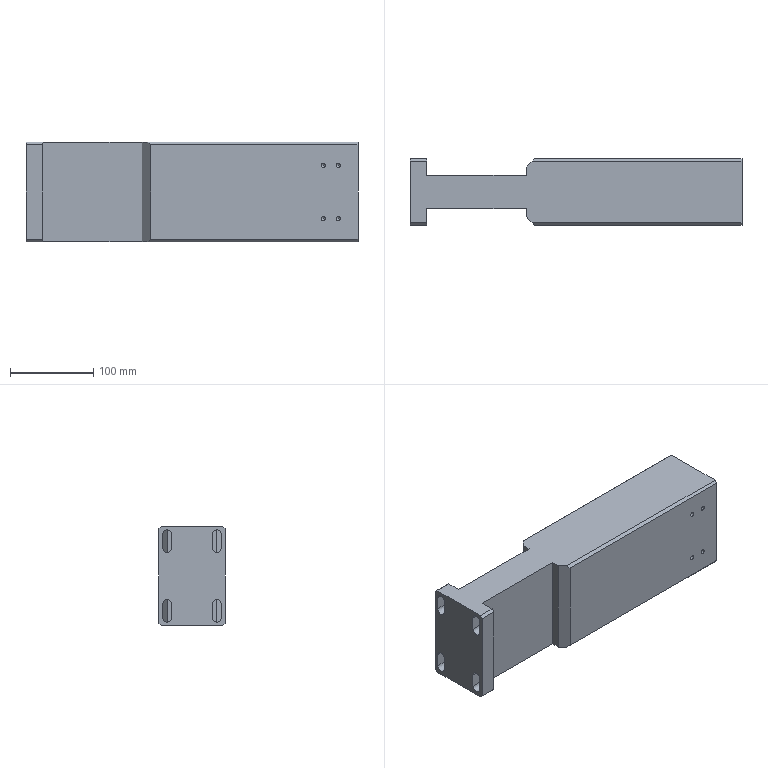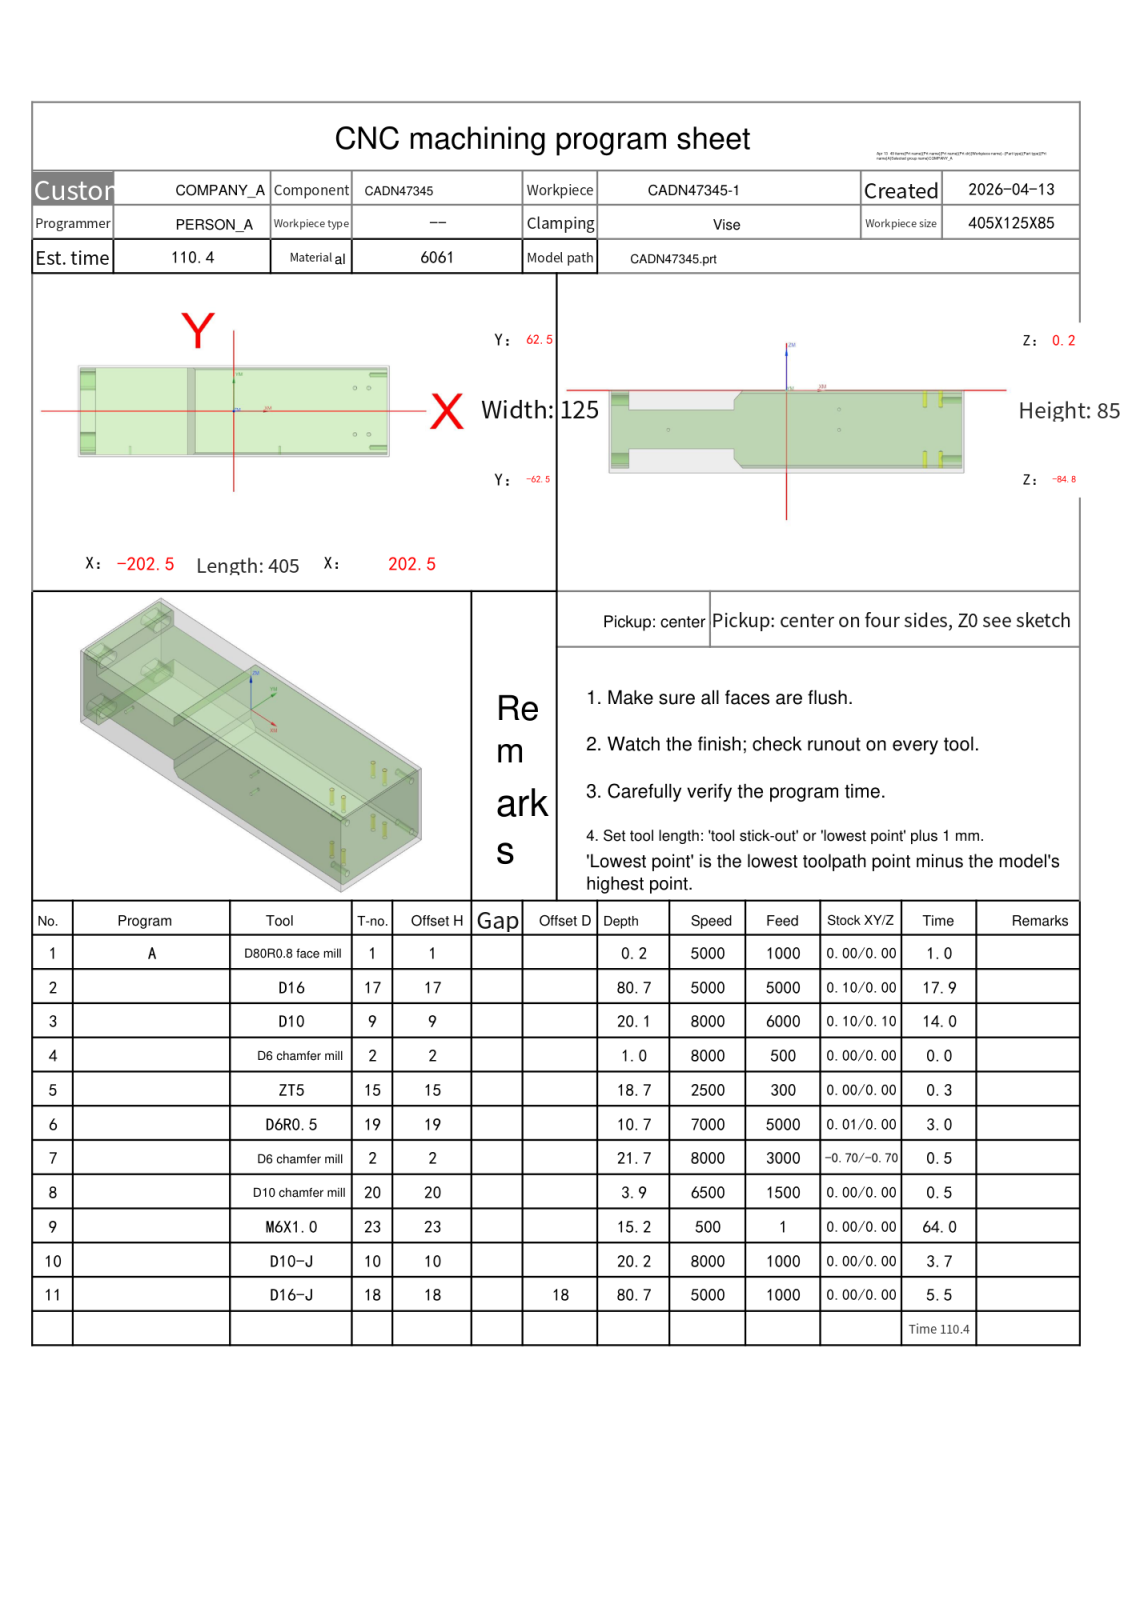NC program | NX | posted by the shop | part box 400 x 80 x 120 mm
Lines 1 to 710 of 5986:
%
O0001
(Machine time: 172.73 MIN)
(===Total Tool:10===)
(T1=D80R0.8 face mill D=80.  R=0.8  D-  H01 Z=0.    )
(T17=D16    D=16.  R=0.   D-  H17 Z=-80.5 )
(T9=D10     D=10.  R=0.   D-  H09 Z=-19.9 )
(T2=D6 chamfer mill   D=6.   R=0.   D-  H02 Z=-21.5 )
(T15=ZT5    D=5.   DR_a=118 D-  H15 Z=-18.5 )
(T19=D6R0.5 D=6.   R=0.5  D-  H19 Z=-10.5 )
(T20=D10 chamfer mill D=10.  R=0.  D-  H20 Z=-3.7  )
(T23=M6X1.0 D=5.   DR_a=180 D-  H23 Z=-15.  )
(T10=D10-J  D=10.  R=0.   D10 H10 Z=-20.  )
(T18=D16-J  D=16.  R=0.   D18 H18 Z=-80.5 )
G80 G90 G17 G49 G40
G91 G28 Z0
M01
N1 T01 M06
(D80R0.8 face mill  D=80. R=0.8 H=01 ce=0.00 di=0.00)
G00 G90 G54 X245. Y-33.333 M03 S5000
G43 H01 Z20.
M08
Z2.
G01 Z0.0 F1000.
X240.
X-240.
Y33.333
X240.
X245.
Z2.
G00 Z20.
G91 G28 Z0.0
M05
M09
G91 G28 Z0.0
M01
N2 T17 M06
(D16  D=16. R=0. H=17 ce=0.10 di=0.00)
G00 G90 G54 X0.0 Y68.1 M03 S5000
G43 H17 Z20.
M08
Z.5
G01 X200. Z.317 F5000.
G02 X208.1 Y60. Z.305 I0.0 J-8.1
G01 Y-60. Z.195
G02 X200. Y-68.1 Z.183 I-8.1 J0.0
G01 X-200. Z-.183
G02 X-208.1 Y-60. Z-.195 I0.0 J8.1
G01 Y60. Z-.305
G02 X-200. Y68.1 Z-.317 I8.1 J0.0
G01 X200. Z-.683
G02 X208.1 Y60. Z-.695 I0.0 J-8.1
G01 Y-60. Z-.805
G02 X200. Y-68.1 Z-.817 I-8.1 J0.0
G01 X-200. Z-1.183
G02 X-208.1 Y-60. Z-1.195 I0.0 J8.1
G01 Y60. Z-1.305
G02 X-200. Y68.1 Z-1.317 I8.1 J0.0
G01 X200. Z-1.683
G02 X208.1 Y60. Z-1.695 I0.0 J-8.1
G01 Y-60. Z-1.805
G02 X200. Y-68.1 Z-1.817 I-8.1 J0.0
G01 X-200. Z-2.183
G02 X-208.1 Y-60. Z-2.195 I0.0 J8.1
G01 Y60. Z-2.305
G02 X-200. Y68.1 Z-2.317 I8.1 J0.0
G01 X200. Z-2.683
G02 X208.1 Y60. Z-2.695 I0.0 J-8.1
G01 Y-60. Z-2.805
G02 X200. Y-68.1 Z-2.817 I-8.1 J0.0
G01 X-200. Z-3.183
G02 X-208.1 Y-60. Z-3.195 I0.0 J8.1
G01 Y60. Z-3.305
G02 X-200. Y68.1 Z-3.317 I8.1 J0.0
G01 X200. Z-3.683
G02 X208.1 Y60. Z-3.695 I0.0 J-8.1
G01 Y-60. Z-3.805
G02 X200. Y-68.1 Z-3.817 I-8.1 J0.0
G01 X-200. Z-4.183
G02 X-208.1 Y-60. Z-4.195 I0.0 J8.1
G01 Y60. Z-4.305
G02 X-200. Y68.1 Z-4.317 I8.1 J0.0
G01 X200. Z-4.683
G02 X208.1 Y60. Z-4.695 I0.0 J-8.1
G01 Y-60. Z-4.805
G02 X200. Y-68.1 Z-4.817 I-8.1 J0.0
G01 X-200. Z-5.183
G02 X-208.1 Y-60. Z-5.195 I0.0 J8.1
G01 Y60. Z-5.305
G02 X-200. Y68.1 Z-5.317 I8.1 J0.0
G01 X200. Z-5.683
G02 X208.1 Y60. Z-5.695 I0.0 J-8.1
G01 Y-60. Z-5.805
G02 X200. Y-68.1 Z-5.817 I-8.1 J0.0
G01 X-200. Z-6.183
G02 X-208.1 Y-60. Z-6.195 I0.0 J8.1
G01 Y60. Z-6.305
G02 X-200. Y68.1 Z-6.317 I8.1 J0.0
G01 X200. Z-6.683
G02 X208.1 Y60. Z-6.695 I0.0 J-8.1
G01 Y-60. Z-6.805
G02 X200. Y-68.1 Z-6.817 I-8.1 J0.0
G01 X-200. Z-7.183
G02 X-208.1 Y-60. Z-7.195 I0.0 J8.1
G01 Y60. Z-7.305
G02 X-200. Y68.1 Z-7.317 I8.1 J0.0
G01 X200. Z-7.683
G02 X208.1 Y60. Z-7.695 I0.0 J-8.1
G01 Y-60. Z-7.805
G02 X200. Y-68.1 Z-7.817 I-8.1 J0.0
G01 X-200. Z-8.183
G02 X-208.1 Y-60. Z-8.195 I0.0 J8.1
G01 Y60. Z-8.305
G02 X-200. Y68.1 Z-8.317 I8.1 J0.0
G01 X200. Z-8.683
G02 X208.1 Y60. Z-8.695 I0.0 J-8.1
G01 Y-60. Z-8.805
G02 X200. Y-68.1 Z-8.817 I-8.1 J0.0
G01 X-200. Z-9.183
G02 X-208.1 Y-60. Z-9.195 I0.0 J8.1
G01 Y60. Z-9.305
G02 X-200. Y68.1 Z-9.317 I8.1 J0.0
G01 X200. Z-9.683
G02 X208.1 Y60. Z-9.695 I0.0 J-8.1
G01 Y-60. Z-9.805
G02 X200. Y-68.1 Z-9.817 I-8.1 J0.0
G01 X-200. Z-10.183
G02 X-208.1 Y-60. Z-10.195 I0.0 J8.1
G01 Y60. Z-10.305
G02 X-200. Y68.1 Z-10.317 I8.1 J0.0
G01 X200. Z-10.683
G02 X208.1 Y60. Z-10.695 I0.0 J-8.1
G01 Y-60. Z-10.805
G02 X200. Y-68.1 Z-10.817 I-8.1 J0.0
G01 X-200. Z-11.183
G02 X-208.1 Y-60. Z-11.195 I0.0 J8.1
G01 Y60. Z-11.305
G02 X-200. Y68.1 Z-11.317 I8.1 J0.0
G01 X200. Z-11.683
G02 X208.1 Y60. Z-11.695 I0.0 J-8.1
G01 Y-60. Z-11.805
G02 X200. Y-68.1 Z-11.817 I-8.1 J0.0
G01 X-200. Z-12.183
G02 X-208.1 Y-60. Z-12.195 I0.0 J8.1
G01 Y60. Z-12.305
G02 X-200. Y68.1 Z-12.317 I8.1 J0.0
G01 X200. Z-12.683
G02 X208.1 Y60. Z-12.695 I0.0 J-8.1
G01 Y-60. Z-12.805
G02 X200. Y-68.1 Z-12.817 I-8.1 J0.0
G01 X-200. Z-13.183
G02 X-208.1 Y-60. Z-13.195 I0.0 J8.1
G01 Y60. Z-13.305
G02 X-200. Y68.1 Z-13.317 I8.1 J0.0
G01 X200. Z-13.683
G02 X208.1 Y60. Z-13.695 I0.0 J-8.1
G01 Y-60. Z-13.805
G02 X200. Y-68.1 Z-13.817 I-8.1 J0.0
G01 X-200. Z-14.183
G02 X-208.1 Y-60. Z-14.195 I0.0 J8.1
G01 Y60. Z-14.305
G02 X-200. Y68.1 Z-14.317 I8.1 J0.0
G01 X200. Z-14.683
G02 X208.1 Y60. Z-14.695 I0.0 J-8.1
G01 Y-60. Z-14.805
G02 X200. Y-68.1 Z-14.817 I-8.1 J0.0
G01 X-200. Z-15.183
G02 X-208.1 Y-60. Z-15.195 I0.0 J8.1
G01 Y60. Z-15.305
G02 X-200. Y68.1 Z-15.317 I8.1 J0.0
G01 X200. Z-15.683
G02 X208.1 Y60. Z-15.695 I0.0 J-8.1
G01 Y-60. Z-15.805
G02 X200. Y-68.1 Z-15.817 I-8.1 J0.0
G01 X-200. Z-16.183
G02 X-208.1 Y-60. Z-16.195 I0.0 J8.1
G01 Y60. Z-16.305
G02 X-200. Y68.1 Z-16.317 I8.1 J0.0
G01 X200. Z-16.683
G02 X208.1 Y60. Z-16.695 I0.0 J-8.1
G01 Y-60. Z-16.805
G02 X200. Y-68.1 Z-16.817 I-8.1 J0.0
G01 X-200. Z-17.183
G02 X-208.1 Y-60. Z-17.195 I0.0 J8.1
G01 Y60. Z-17.305
G02 X-200. Y68.1 Z-17.317 I8.1 J0.0
G01 X200. Z-17.683
G02 X208.1 Y60. Z-17.695 I0.0 J-8.1
G01 Y-60. Z-17.805
G02 X200. Y-68.1 Z-17.817 I-8.1 J0.0
G01 X-200. Z-18.183
G02 X-208.1 Y-60. Z-18.195 I0.0 J8.1
G01 Y60. Z-18.305
G02 X-200. Y68.1 Z-18.317 I8.1 J0.0
G01 X200. Z-18.683
G02 X208.1 Y60. Z-18.695 I0.0 J-8.1
G01 Y-60. Z-18.805
G02 X200. Y-68.1 Z-18.817 I-8.1 J0.0
G01 X-200. Z-19.183
G02 X-208.1 Y-60. Z-19.195 I0.0 J8.1
G01 Y60. Z-19.305
G02 X-200. Y68.1 Z-19.317 I8.1 J0.0
G01 X200. Z-19.683
G02 X208.1 Y60. Z-19.695 I0.0 J-8.1
G01 Y-60. Z-19.805
G02 X200. Y-68.1 Z-19.817 I-8.1 J0.0
G01 X-200. Z-20.183
G02 X-208.1 Y-60. Z-20.195 I0.0 J8.1
G01 Y60. Z-20.305
G02 X-200. Y68.1 Z-20.317 I8.1 J0.0
G01 X200. Z-20.683
G02 X208.1 Y60. Z-20.695 I0.0 J-8.1
G01 Y-60. Z-20.805
G02 X200. Y-68.1 Z-20.817 I-8.1 J0.0
G01 X-200. Z-21.183
G02 X-208.1 Y-60. Z-21.195 I0.0 J8.1
G01 Y60. Z-21.305
G02 X-200. Y68.1 Z-21.317 I8.1 J0.0
G01 X200. Z-21.683
G02 X208.1 Y60. Z-21.695 I0.0 J-8.1
G01 Y-60. Z-21.805
G02 X200. Y-68.1 Z-21.817 I-8.1 J0.0
G01 X-200. Z-22.183
G02 X-208.1 Y-60. Z-22.195 I0.0 J8.1
G01 Y60. Z-22.305
G02 X-200. Y68.1 Z-22.317 I8.1 J0.0
G01 X200. Z-22.683
G02 X208.1 Y60. Z-22.695 I0.0 J-8.1
G01 Y-60. Z-22.805
G02 X200. Y-68.1 Z-22.817 I-8.1 J0.0
G01 X-200. Z-23.183
G02 X-208.1 Y-60. Z-23.195 I0.0 J8.1
G01 Y60. Z-23.305
G02 X-200. Y68.1 Z-23.317 I8.1 J0.0
G01 X200. Z-23.683
G02 X208.1 Y60. Z-23.695 I0.0 J-8.1
G01 Y-60. Z-23.805
G02 X200. Y-68.1 Z-23.817 I-8.1 J0.0
G01 X-200. Z-24.183
G02 X-208.1 Y-60. Z-24.195 I0.0 J8.1
G01 Y60. Z-24.305
G02 X-200. Y68.1 Z-24.317 I8.1 J0.0
G01 X200. Z-24.683
G02 X208.1 Y60. Z-24.695 I0.0 J-8.1
G01 Y-60. Z-24.805
G02 X200. Y-68.1 Z-24.817 I-8.1 J0.0
G01 X-200. Z-25.183
G02 X-208.1 Y-60. Z-25.195 I0.0 J8.1
G01 Y60. Z-25.305
G02 X-200. Y68.1 Z-25.317 I8.1 J0.0
G01 X200. Z-25.683
G02 X208.1 Y60. Z-25.695 I0.0 J-8.1
G01 Y-60. Z-25.805
G02 X200. Y-68.1 Z-25.817 I-8.1 J0.0
G01 X-200. Z-26.183
G02 X-208.1 Y-60. Z-26.195 I0.0 J8.1
G01 Y60. Z-26.305
G02 X-200. Y68.1 Z-26.317 I8.1 J0.0
G01 X200. Z-26.683
G02 X208.1 Y60. Z-26.695 I0.0 J-8.1
G01 Y-60. Z-26.805
G02 X200. Y-68.1 Z-26.817 I-8.1 J0.0
G01 X-200. Z-27.183
G02 X-208.1 Y-60. Z-27.195 I0.0 J8.1
G01 Y60. Z-27.305
G02 X-200. Y68.1 Z-27.317 I8.1 J0.0
G01 X200. Z-27.683
G02 X208.1 Y60. Z-27.695 I0.0 J-8.1
G01 Y-60. Z-27.805
G02 X200. Y-68.1 Z-27.817 I-8.1 J0.0
G01 X-200. Z-28.183
G02 X-208.1 Y-60. Z-28.195 I0.0 J8.1
G01 Y60. Z-28.305
G02 X-200. Y68.1 Z-28.317 I8.1 J0.0
G01 X200. Z-28.683
G02 X208.1 Y60. Z-28.695 I0.0 J-8.1
G01 Y-60. Z-28.805
G02 X200. Y-68.1 Z-28.817 I-8.1 J0.0
G01 X-200. Z-29.183
G02 X-208.1 Y-60. Z-29.195 I0.0 J8.1
G01 Y60. Z-29.305
G02 X-200. Y68.1 Z-29.317 I8.1 J0.0
G01 X200. Z-29.683
G02 X208.1 Y60. Z-29.695 I0.0 J-8.1
G01 Y-60. Z-29.805
G02 X200. Y-68.1 Z-29.817 I-8.1 J0.0
G01 X-200. Z-30.183
G02 X-208.1 Y-60. Z-30.195 I0.0 J8.1
G01 Y60. Z-30.305
G02 X-200. Y68.1 Z-30.317 I8.1 J0.0
G01 X200. Z-30.683
G02 X208.1 Y60. Z-30.695 I0.0 J-8.1
G01 Y-60. Z-30.805
G02 X200. Y-68.1 Z-30.817 I-8.1 J0.0
G01 X-200. Z-31.183
G02 X-208.1 Y-60. Z-31.195 I0.0 J8.1
G01 Y60. Z-31.305
G02 X-200. Y68.1 Z-31.317 I8.1 J0.0
G01 X200. Z-31.683
G02 X208.1 Y60. Z-31.695 I0.0 J-8.1
G01 Y-60. Z-31.805
G02 X200. Y-68.1 Z-31.817 I-8.1 J0.0
G01 X-200. Z-32.183
G02 X-208.1 Y-60. Z-32.195 I0.0 J8.1
G01 Y60. Z-32.305
G02 X-200. Y68.1 Z-32.317 I8.1 J0.0
G01 X200. Z-32.683
G02 X208.1 Y60. Z-32.695 I0.0 J-8.1
G01 Y-60. Z-32.805
G02 X200. Y-68.1 Z-32.817 I-8.1 J0.0
G01 X-200. Z-33.183
G02 X-208.1 Y-60. Z-33.195 I0.0 J8.1
G01 Y60. Z-33.305
G02 X-200. Y68.1 Z-33.317 I8.1 J0.0
G01 X200. Z-33.683
G02 X208.1 Y60. Z-33.695 I0.0 J-8.1
G01 Y-60. Z-33.805
G02 X200. Y-68.1 Z-33.817 I-8.1 J0.0
G01 X-200. Z-34.183
G02 X-208.1 Y-60. Z-34.195 I0.0 J8.1
G01 Y60. Z-34.305
G02 X-200. Y68.1 Z-34.317 I8.1 J0.0
G01 X200. Z-34.683
G02 X208.1 Y60. Z-34.695 I0.0 J-8.1
G01 Y-60. Z-34.805
G02 X200. Y-68.1 Z-34.817 I-8.1 J0.0
G01 X-200. Z-35.183
G02 X-208.1 Y-60. Z-35.195 I0.0 J8.1
G01 Y60. Z-35.305
G02 X-200. Y68.1 Z-35.317 I8.1 J0.0
G01 X200. Z-35.683
G02 X208.1 Y60. Z-35.695 I0.0 J-8.1
G01 Y-60. Z-35.805
G02 X200. Y-68.1 Z-35.817 I-8.1 J0.0
G01 X-200. Z-36.183
G02 X-208.1 Y-60. Z-36.195 I0.0 J8.1
G01 Y60. Z-36.305
G02 X-200. Y68.1 Z-36.317 I8.1 J0.0
G01 X200. Z-36.683
G02 X208.1 Y60. Z-36.695 I0.0 J-8.1
G01 Y-60. Z-36.805
G02 X200. Y-68.1 Z-36.817 I-8.1 J0.0
G01 X-200. Z-37.183
G02 X-208.1 Y-60. Z-37.195 I0.0 J8.1
G01 Y60. Z-37.305
G02 X-200. Y68.1 Z-37.317 I8.1 J0.0
G01 X200. Z-37.683
G02 X208.1 Y60. Z-37.695 I0.0 J-8.1
G01 Y-60. Z-37.805
G02 X200. Y-68.1 Z-37.817 I-8.1 J0.0
G01 X-200. Z-38.183
G02 X-208.1 Y-60. Z-38.195 I0.0 J8.1
G01 Y60. Z-38.305
G02 X-200. Y68.1 Z-38.317 I8.1 J0.0
G01 X200. Z-38.683
G02 X208.1 Y60. Z-38.695 I0.0 J-8.1
G01 Y-60. Z-38.805
G02 X200. Y-68.1 Z-38.817 I-8.1 J0.0
G01 X-200. Z-39.183
G02 X-208.1 Y-60. Z-39.195 I0.0 J8.1
G01 Y60. Z-39.305
G02 X-200. Y68.1 Z-39.317 I8.1 J0.0
G01 X200. Z-39.683
G02 X208.1 Y60. Z-39.695 I0.0 J-8.1
G01 Y-60. Z-39.805
G02 X200. Y-68.1 Z-39.817 I-8.1 J0.0
G01 X-200. Z-40.183
G02 X-208.1 Y-60. Z-40.195 I0.0 J8.1
G01 Y60. Z-40.305
G02 X-200. Y68.1 Z-40.317 I8.1 J0.0
G01 X200. Z-40.683
G02 X208.1 Y60. Z-40.695 I0.0 J-8.1
G01 Y-60. Z-40.805
G02 X200. Y-68.1 Z-40.817 I-8.1 J0.0
G01 X-200. Z-41.183
G02 X-208.1 Y-60. Z-41.195 I0.0 J8.1
G01 Y60. Z-41.305
G02 X-200. Y68.1 Z-41.317 I8.1 J0.0
G01 X200. Z-41.683
G02 X208.1 Y60. Z-41.695 I0.0 J-8.1
G01 Y-60. Z-41.805
G02 X200. Y-68.1 Z-41.817 I-8.1 J0.0
G01 X-200. Z-42.183
G02 X-208.1 Y-60. Z-42.195 I0.0 J8.1
G01 Y60. Z-42.305
G02 X-200. Y68.1 Z-42.317 I8.1 J0.0
G01 X200. Z-42.683
G02 X208.1 Y60. Z-42.695 I0.0 J-8.1
G01 Y-60. Z-42.805
G02 X200. Y-68.1 Z-42.817 I-8.1 J0.0
G01 X-200. Z-43.183
G02 X-208.1 Y-60. Z-43.195 I0.0 J8.1
G01 Y60. Z-43.305
G02 X-200. Y68.1 Z-43.317 I8.1 J0.0
G01 X200. Z-43.683
G02 X208.1 Y60. Z-43.695 I0.0 J-8.1
G01 Y-60. Z-43.805
G02 X200. Y-68.1 Z-43.817 I-8.1 J0.0
G01 X-200. Z-44.183
G02 X-208.1 Y-60. Z-44.195 I0.0 J8.1
G01 Y60. Z-44.305
G02 X-200. Y68.1 Z-44.317 I8.1 J0.0
G01 X200. Z-44.683
G02 X208.1 Y60. Z-44.695 I0.0 J-8.1
G01 Y-60. Z-44.805
G02 X200. Y-68.1 Z-44.817 I-8.1 J0.0
G01 X-200. Z-45.183
G02 X-208.1 Y-60. Z-45.195 I0.0 J8.1
G01 Y60. Z-45.305
G02 X-200. Y68.1 Z-45.317 I8.1 J0.0
G01 X200. Z-45.683
G02 X208.1 Y60. Z-45.695 I0.0 J-8.1
G01 Y-60. Z-45.805
G02 X200. Y-68.1 Z-45.817 I-8.1 J0.0
G01 X-200. Z-46.183
G02 X-208.1 Y-60. Z-46.195 I0.0 J8.1
G01 Y60. Z-46.305
G02 X-200. Y68.1 Z-46.317 I8.1 J0.0
G01 X200. Z-46.683
G02 X208.1 Y60. Z-46.695 I0.0 J-8.1
G01 Y-60. Z-46.805
G02 X200. Y-68.1 Z-46.817 I-8.1 J0.0
G01 X-200. Z-47.183
G02 X-208.1 Y-60. Z-47.195 I0.0 J8.1
G01 Y60. Z-47.305
G02 X-200. Y68.1 Z-47.317 I8.1 J0.0
G01 X200. Z-47.683
G02 X208.1 Y60. Z-47.695 I0.0 J-8.1
G01 Y-60. Z-47.805
G02 X200. Y-68.1 Z-47.817 I-8.1 J0.0
G01 X-200. Z-48.183
G02 X-208.1 Y-60. Z-48.195 I0.0 J8.1
G01 Y60. Z-48.305
G02 X-200. Y68.1 Z-48.317 I8.1 J0.0
G01 X200. Z-48.683
G02 X208.1 Y60. Z-48.695 I0.0 J-8.1
G01 Y-60. Z-48.805
G02 X200. Y-68.1 Z-48.817 I-8.1 J0.0
G01 X-200. Z-49.183
G02 X-208.1 Y-60. Z-49.195 I0.0 J8.1
G01 Y60. Z-49.305
G02 X-200. Y68.1 Z-49.317 I8.1 J0.0
G01 X200. Z-49.683
G02 X208.1 Y60. Z-49.695 I0.0 J-8.1
G01 Y-60. Z-49.805
G02 X200. Y-68.1 Z-49.817 I-8.1 J0.0
G01 X-200. Z-50.183
G02 X-208.1 Y-60. Z-50.195 I0.0 J8.1
G01 Y60. Z-50.305
G02 X-200. Y68.1 Z-50.317 I8.1 J0.0
G01 X200. Z-50.683
G02 X208.1 Y60. Z-50.695 I0.0 J-8.1
G01 Y-60. Z-50.805
G02 X200. Y-68.1 Z-50.817 I-8.1 J0.0
G01 X-200. Z-51.183
G02 X-208.1 Y-60. Z-51.195 I0.0 J8.1
G01 Y60. Z-51.305
G02 X-200. Y68.1 Z-51.317 I8.1 J0.0
G01 X200. Z-51.683
G02 X208.1 Y60. Z-51.695 I0.0 J-8.1
G01 Y-60. Z-51.805
G02 X200. Y-68.1 Z-51.817 I-8.1 J0.0
G01 X-200. Z-52.183
G02 X-208.1 Y-60. Z-52.195 I0.0 J8.1
G01 Y60. Z-52.305
G02 X-200. Y68.1 Z-52.317 I8.1 J0.0
G01 X200. Z-52.683
G02 X208.1 Y60. Z-52.695 I0.0 J-8.1
G01 Y-60. Z-52.805
G02 X200. Y-68.1 Z-52.817 I-8.1 J0.0
G01 X-200. Z-53.183
G02 X-208.1 Y-60. Z-53.195 I0.0 J8.1
G01 Y60. Z-53.305
G02 X-200. Y68.1 Z-53.317 I8.1 J0.0
G01 X200. Z-53.683
G02 X208.1 Y60. Z-53.695 I0.0 J-8.1
G01 Y-60. Z-53.805
G02 X200. Y-68.1 Z-53.817 I-8.1 J0.0
G01 X-200. Z-54.183
G02 X-208.1 Y-60. Z-54.195 I0.0 J8.1
G01 Y60. Z-54.305
G02 X-200. Y68.1 Z-54.317 I8.1 J0.0
G01 X200. Z-54.683
G02 X208.1 Y60. Z-54.695 I0.0 J-8.1
G01 Y-60. Z-54.805
G02 X200. Y-68.1 Z-54.817 I-8.1 J0.0
G01 X-200. Z-55.183
G02 X-208.1 Y-60. Z-55.195 I0.0 J8.1
G01 Y60. Z-55.305
G02 X-200. Y68.1 Z-55.317 I8.1 J0.0
G01 X200. Z-55.683
G02 X208.1 Y60. Z-55.695 I0.0 J-8.1
G01 Y-60. Z-55.805
G02 X200. Y-68.1 Z-55.817 I-8.1 J0.0
G01 X-200. Z-56.183
G02 X-208.1 Y-60. Z-56.195 I0.0 J8.1
G01 Y60. Z-56.305
G02 X-200. Y68.1 Z-56.317 I8.1 J0.0
G01 X200. Z-56.683
G02 X208.1 Y60. Z-56.695 I0.0 J-8.1
G01 Y-60. Z-56.805
G02 X200. Y-68.1 Z-56.817 I-8.1 J0.0
G01 X-200. Z-57.183
G02 X-208.1 Y-60. Z-57.195 I0.0 J8.1
G01 Y60. Z-57.305
G02 X-200. Y68.1 Z-57.317 I8.1 J0.0
G01 X200. Z-57.683
G02 X208.1 Y60. Z-57.695 I0.0 J-8.1
G01 Y-60. Z-57.805
G02 X200. Y-68.1 Z-57.817 I-8.1 J0.0
G01 X-200. Z-58.183
G02 X-208.1 Y-60. Z-58.195 I0.0 J8.1
G01 Y60. Z-58.305
G02 X-200. Y68.1 Z-58.317 I8.1 J0.0
G01 X200. Z-58.683
G02 X208.1 Y60. Z-58.695 I0.0 J-8.1
G01 Y-60. Z-58.805
G02 X200. Y-68.1 Z-58.817 I-8.1 J0.0
G01 X-200. Z-59.183
G02 X-208.1 Y-60. Z-59.195 I0.0 J8.1
G01 Y60. Z-59.305
G02 X-200. Y68.1 Z-59.317 I8.1 J0.0
G01 X200. Z-59.683
G02 X208.1 Y60. Z-59.695 I0.0 J-8.1
G01 Y-60. Z-59.805
G02 X200. Y-68.1 Z-59.817 I-8.1 J0.0
G01 X-200. Z-60.183
G02 X-208.1 Y-60. Z-60.195 I0.0 J8.1
G01 Y60. Z-60.305
G02 X-200. Y68.1 Z-60.317 I8.1 J0.0
G01 X200. Z-60.683
G02 X208.1 Y60. Z-60.695 I0.0 J-8.1
G01 Y-60. Z-60.805
G02 X200. Y-68.1 Z-60.817 I-8.1 J0.0
G01 X-200. Z-61.183
G02 X-208.1 Y-60. Z-61.195 I0.0 J8.1
G01 Y60. Z-61.305
G02 X-200. Y68.1 Z-61.317 I8.1 J0.0
G01 X200. Z-61.683
G02 X208.1 Y60. Z-61.695 I0.0 J-8.1
G01 Y-60. Z-61.805
G02 X200. Y-68.1 Z-61.817 I-8.1 J0.0
G01 X-200. Z-62.183
G02 X-208.1 Y-60. Z-62.195 I0.0 J8.1
G01 Y60. Z-62.305
G02 X-200. Y68.1 Z-62.317 I8.1 J0.0
G01 X200. Z-62.683
G02 X208.1 Y60. Z-62.695 I0.0 J-8.1
G01 Y-60. Z-62.805
G02 X200. Y-68.1 Z-62.817 I-8.1 J0.0
G01 X-200. Z-63.183
G02 X-208.1 Y-60. Z-63.195 I0.0 J8.1
G01 Y60. Z-63.305
G02 X-200. Y68.1 Z-63.317 I8.1 J0.0
G01 X200. Z-63.683
G02 X208.1 Y60. Z-63.695 I0.0 J-8.1
G01 Y-60. Z-63.805
G02 X200. Y-68.1 Z-63.817 I-8.1 J0.0
G01 X-200. Z-64.183
G02 X-208.1 Y-60. Z-64.195 I0.0 J8.1
G01 Y60. Z-64.305
G02 X-200. Y68.1 Z-64.317 I8.1 J0.0
G01 X200. Z-64.683
G02 X208.1 Y60. Z-64.695 I0.0 J-8.1
G01 Y-60. Z-64.805
G02 X200. Y-68.1 Z-64.817 I-8.1 J0.0
G01 X-200. Z-65.183
G02 X-208.1 Y-60. Z-65.195 I0.0 J8.1
G01 Y60. Z-65.305
G02 X-200. Y68.1 Z-65.317 I8.1 J0.0
G01 X200. Z-65.683
G02 X208.1 Y60. Z-65.695 I0.0 J-8.1
G01 Y-60. Z-65.805
G02 X200. Y-68.1 Z-65.817 I-8.1 J0.0
G01 X-200. Z-66.183
G02 X-208.1 Y-60. Z-66.195 I0.0 J8.1
G01 Y60. Z-66.305
G02 X-200. Y68.1 Z-66.317 I8.1 J0.0
G01 X200. Z-66.683
G02 X208.1 Y60. Z-66.695 I0.0 J-8.1
G01 Y-60. Z-66.805
G02 X200. Y-68.1 Z-66.817 I-8.1 J0.0
G01 X-200. Z-67.183
G02 X-208.1 Y-60. Z-67.195 I0.0 J8.1
G01 Y60. Z-67.305
G02 X-200. Y68.1 Z-67.317 I8.1 J0.0
G01 X200. Z-67.683
G02 X208.1 Y60. Z-67.695 I0.0 J-8.1
G01 Y-60. Z-67.805
G02 X200. Y-68.1 Z-67.817 I-8.1 J0.0
G01 X-200. Z-68.183
G02 X-208.1 Y-60. Z-68.195 I0.0 J8.1
G01 Y60. Z-68.305
G02 X-200. Y68.1 Z-68.317 I8.1 J0.0
G01 X200. Z-68.683
G02 X208.1 Y60. Z-68.695 I0.0 J-8.1
G01 Y-60. Z-68.805
G02 X200. Y-68.1 Z-68.817 I-8.1 J0.0
G01 X-200. Z-69.183
G02 X-208.1 Y-60. Z-69.195 I0.0 J8.1
G01 Y60. Z-69.305
G02 X-200. Y68.1 Z-69.317 I8.1 J0.0
G01 X200. Z-69.683
G02 X208.1 Y60. Z-69.695 I0.0 J-8.1
G01 Y-60. Z-69.805
G02 X200. Y-68.1 Z-69.817 I-8.1 J0.0
G01 X-200. Z-70.183
G02 X-208.1 Y-60. Z-70.195 I0.0 J8.1
G01 Y60. Z-70.305
G02 X-200. Y68.1 Z-70.317 I8.1 J0.0
G01 X200. Z-70.683
G02 X208.1 Y60. Z-70.695 I0.0 J-8.1
G01 Y-60. Z-70.805
G02 X200. Y-68.1 Z-70.817 I-8.1 J0.0
G01 X-200. Z-71.183
G02 X-208.1 Y-60. Z-71.195 I0.0 J8.1
G01 Y60. Z-71.305
G02 X-200. Y68.1 Z-71.317 I8.1 J0.0
G01 X200. Z-71.683
G02 X208.1 Y60. Z-71.695 I0.0 J-8.1
G01 Y-60. Z-71.805
G02 X200. Y-68.1 Z-71.817 I-8.1 J0.0
G01 X-200. Z-72.183
G02 X-208.1 Y-60. Z-72.195 I0.0 J8.1
G01 Y60. Z-72.305
G02 X-200. Y68.1 Z-72.317 I8.1 J0.0
G01 X200. Z-72.683
G02 X208.1 Y60. Z-72.695 I0.0 J-8.1
G01 Y-60. Z-72.805
G02 X200. Y-68.1 Z-72.817 I-8.1 J0.0
G01 X-200. Z-73.183
G02 X-208.1 Y-60. Z-73.195 I0.0 J8.1
G01 Y60. Z-73.305
G02 X-200. Y68.1 Z-73.317 I8.1 J0.0
G01 X200. Z-73.683
G02 X208.1 Y60. Z-73.695 I0.0 J-8.1
G01 Y-60. Z-73.805
G02 X200. Y-68.1 Z-73.817 I-8.1 J0.0
G01 X-200. Z-74.183
G02 X-208.1 Y-60. Z-74.195 I0.0 J8.1
G01 Y60. Z-74.305
G02 X-200. Y68.1 Z-74.317 I8.1 J0.0
G01 X200. Z-74.683
G02 X208.1 Y60. Z-74.695 I0.0 J-8.1
G01 Y-60. Z-74.805
G02 X200. Y-68.1 Z-74.817 I-8.1 J0.0
G01 X-200. Z-75.183
G02 X-208.1 Y-60. Z-75.195 I0.0 J8.1
G01 Y60. Z-75.305
G02 X-200. Y68.1 Z-75.317 I8.1 J0.0
G01 X200. Z-75.683
G02 X208.1 Y60. Z-75.695 I0.0 J-8.1
G01 Y-60. Z-75.805
G02 X200. Y-68.1 Z-75.817 I-8.1 J0.0
G01 X-200. Z-76.183
G02 X-208.1 Y-60. Z-76.195 I0.0 J8.1
G01 Y60. Z-76.305
G02 X-200. Y68.1 Z-76.317 I8.1 J0.0
G01 X200. Z-76.683
G02 X208.1 Y60. Z-76.695 I0.0 J-8.1
G01 Y-60. Z-76.805
G02 X200. Y-68.1 Z-76.817 I-8.1 J0.0
G01 X-200. Z-77.183
G02 X-208.1 Y-60. Z-77.195 I0.0 J8.1
G01 Y60. Z-77.305
G02 X-200. Y68.1 Z-77.317 I8.1 J0.0
G01 X200. Z-77.683
G02 X208.1 Y60. Z-77.695 I0.0 J-8.1
G01 Y-60. Z-77.805
G02 X200. Y-68.1 Z-77.817 I-8.1 J0.0
G01 X-200. Z-78.183
G02 X-208.1 Y-60. Z-78.195 I0.0 J8.1
G01 Y60. Z-78.305
G02 X-200. Y68.1 Z-78.317 I8.1 J0.0
G01 X200. Z-78.683
G02 X208.1 Y60. Z-78.695 I0.0 J-8.1
G01 Y-60. Z-78.805
G02 X200. Y-68.1 Z-78.817 I-8.1 J0.0
G01 X-200. Z-79.183
G02 X-208.1 Y-60. Z-79.195 I0.0 J8.1
G01 Y60. Z-79.305
G02 X-200. Y68.1 Z-79.317 I8.1 J0.0
G01 X200. Z-79.683
G02 X208.1 Y60. Z-79.695 I0.0 J-8.1
G01 Y-60. Z-79.805
G02 X200. Y-68.1 Z-79.817 I-8.1 J0.0
G01 X-200. Z-80.183
G02 X-208.1 Y-60. Z-80.195 I0.0 J8.1
G01 Y60. Z-80.305
G02 X-200. Y68.1 Z-80.317 I8.1 J0.0
G01 X0.0 Z-80.5
X200.
G02 X208.1 Y60. I0.0 J-8.1
G01 Y-60.
G02 X200. Y-68.1 I-8.1 J0.0
G01 X-200.
G02 X-208.1 Y-60. I0.0 J8.1
G01 Y60.
G02 X-200. Y68.1 I8.1 J0.0
G01 X0.0
X.5
Z-79.5
G00 Z20.
G91 G28 Z0.0
M05
M09
G91 G28 Z0.0
M01